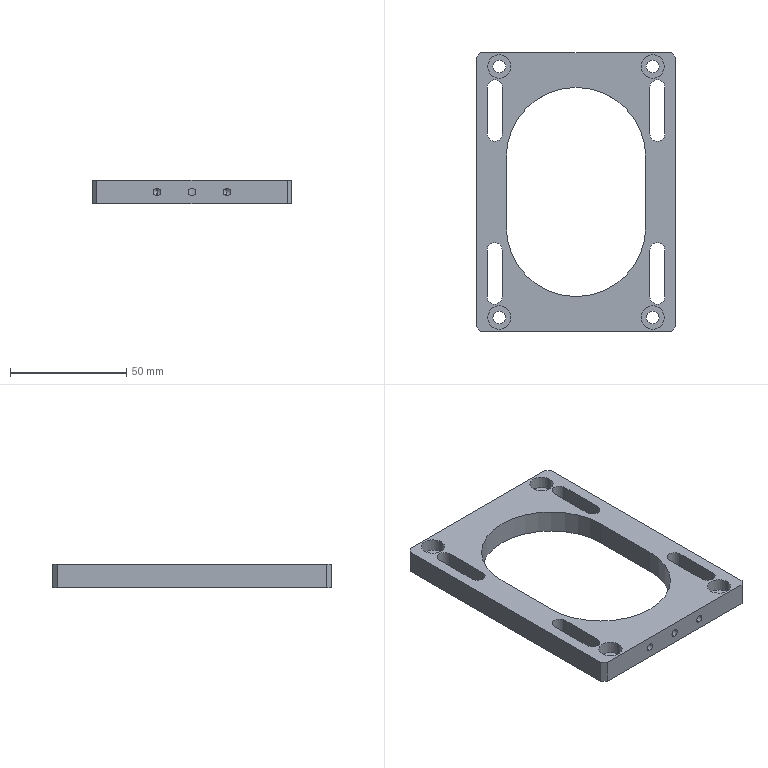Part | STEP file | 11-FG-E03811 | 1 solid | 62 faces | box 86 x 120 x 10 mm | volume 47794 mm3 | cylinder 32 | plane 24 | cone 6 | commonest cylinder face diameters 5.5 x8 6.5 x8 10 x8 3.3 x6 60 x2